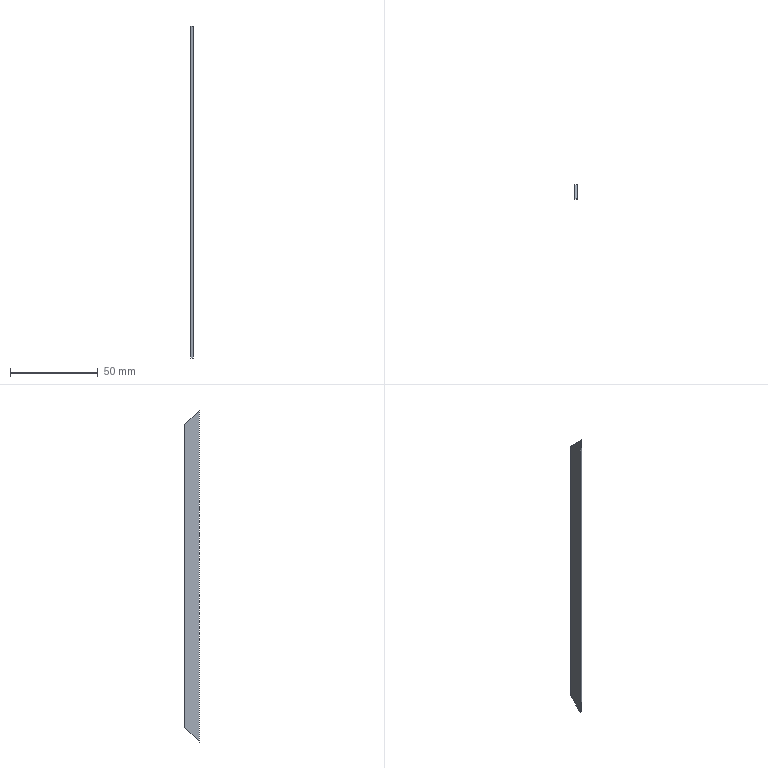Part | NX | features BREP 1 | 1 solid | 6 faces | box 1.5 x 8 x 189.5 mm | volume 2178 mm3 | plane 6
STEP:
#1=CARTESIAN_POINT('',(0.,8.,86.75));
#2=VERTEX_POINT('',#1);
#3=CARTESIAN_POINT('',(0.,8.,-86.75));
#4=VERTEX_POINT('',#3);
#5=CARTESIAN_POINT('',(0.,8.,94.75));
#6=DIRECTION('',(0.,0.,-1.));
#7=VECTOR('',#6,1000.);
#8=LINE('',#5,#7);
#9=EDGE_CURVE('',#2,#4,#8,.T.);
#10=ORIENTED_EDGE('',*,*,#9,.T.);
#11=CARTESIAN_POINT('',(0.,0.,-94.75));
#12=VERTEX_POINT('',#11);
#13=CARTESIAN_POINT('',(0.,8.,-86.75));
#14=DIRECTION('',(0.,-0.7071,-0.7071));
#15=VECTOR('',#14,1000.);
#16=LINE('',#13,#15);
#17=EDGE_CURVE('',#4,#12,#16,.T.);
#18=ORIENTED_EDGE('',*,*,#17,.T.);
#19=CARTESIAN_POINT('',(0.,0.,94.75));
#20=VERTEX_POINT('',#19);
#21=CARTESIAN_POINT('',(0.,0.,94.75));
#22=DIRECTION('',(0.,0.,-1.));
#23=VECTOR('',#22,1000.);
#24=LINE('',#21,#23);
#25=EDGE_CURVE('',#20,#12,#24,.T.);
#26=ORIENTED_EDGE('',*,*,#25,.F.);
#27=CARTESIAN_POINT('',(0.,0.,94.75));
#28=DIRECTION('',(0.,0.7071,-0.7071));
#29=VECTOR('',#28,1000.);
#30=LINE('',#27,#29);
#31=EDGE_CURVE('',#20,#2,#30,.T.);
#32=ORIENTED_EDGE('',*,*,#31,.T.);
#33=EDGE_LOOP('',(#10,#18,#26,#32));
#34=FACE_BOUND('',#33,.T.);
#35=CARTESIAN_POINT('',(0.,0.,94.75));
#36=DIRECTION('',(1.,0.,0.));
#37=DIRECTION('',(0.,1.,0.));
#38=AXIS2_PLACEMENT_3D('',#35,#36,#37);
#39=PLANE('',#38);
#40=ADVANCED_FACE('',(#34),#39,.F.);
#41=CARTESIAN_POINT('',(1.5,0.,-94.75));
#42=VERTEX_POINT('',#41);
#43=CARTESIAN_POINT('',(0.,0.,-94.75));
#44=DIRECTION('',(1.,0.,0.));
#45=VECTOR('',#44,1000.);
#46=LINE('',#43,#45);
#47=EDGE_CURVE('',#12,#42,#46,.T.);
#48=ORIENTED_EDGE('',*,*,#47,.T.);
#49=CARTESIAN_POINT('',(1.5,0.,94.75));
#50=VERTEX_POINT('',#49);
#51=CARTESIAN_POINT('',(1.5,0.,94.75));
#52=DIRECTION('',(0.,0.,-1.));
#53=VECTOR('',#52,1000.);
#54=LINE('',#51,#53);
#55=EDGE_CURVE('',#50,#42,#54,.T.);
#56=ORIENTED_EDGE('',*,*,#55,.F.);
#57=CARTESIAN_POINT('',(0.,0.,94.75));
#58=DIRECTION('',(1.,0.,0.));
#59=VECTOR('',#58,1000.);
#60=LINE('',#57,#59);
#61=EDGE_CURVE('',#20,#50,#60,.T.);
#62=ORIENTED_EDGE('',*,*,#61,.F.);
#63=ORIENTED_EDGE('',*,*,#25,.T.);
#64=EDGE_LOOP('',(#48,#56,#62,#63));
#65=FACE_BOUND('',#64,.T.);
#66=CARTESIAN_POINT('',(0.,0.,94.75));
#67=DIRECTION('',(0.,1.,0.));
#68=DIRECTION('',(1.,0.,0.));
#69=AXIS2_PLACEMENT_3D('',#66,#67,#68);
#70=PLANE('',#69);
#71=ADVANCED_FACE('',(#65),#70,.F.);
#72=ORIENTED_EDGE('',*,*,#55,.T.);
#73=CARTESIAN_POINT('',(1.5,8.,-86.75));
#74=VERTEX_POINT('',#73);
#75=CARTESIAN_POINT('',(1.5,8.,-86.75));
#76=DIRECTION('',(0.,0.7071,0.7071));
#77=VECTOR('',#76,1000.);
#78=LINE('',#75,#77);
#79=EDGE_CURVE('',#42,#74,#78,.T.);
#80=ORIENTED_EDGE('',*,*,#79,.T.);
#81=CARTESIAN_POINT('',(1.5,8.,86.75));
#82=VERTEX_POINT('',#81);
#83=CARTESIAN_POINT('',(1.5,8.,94.75));
#84=DIRECTION('',(0.,0.,-1.));
#85=VECTOR('',#84,1000.);
#86=LINE('',#83,#85);
#87=EDGE_CURVE('',#82,#74,#86,.T.);
#88=ORIENTED_EDGE('',*,*,#87,.F.);
#89=CARTESIAN_POINT('',(1.5,0.,94.75));
#90=DIRECTION('',(0.,-0.7071,0.7071));
#91=VECTOR('',#90,1000.);
#92=LINE('',#89,#91);
#93=EDGE_CURVE('',#82,#50,#92,.T.);
#94=ORIENTED_EDGE('',*,*,#93,.T.);
#95=EDGE_LOOP('',(#72,#80,#88,#94));
#96=FACE_BOUND('',#95,.T.);
#97=CARTESIAN_POINT('',(1.5,0.,94.75));
#98=DIRECTION('',(-1.,0.,0.));
#99=DIRECTION('',(0.,0.,1.));
#100=AXIS2_PLACEMENT_3D('',#97,#98,#99);
#101=PLANE('',#100);
#102=ADVANCED_FACE('',(#96),#101,.F.);
#103=ORIENTED_EDGE('',*,*,#87,.T.);
#104=CARTESIAN_POINT('',(0.,8.,-86.75));
#105=DIRECTION('',(-1.,0.,0.));
#106=VECTOR('',#105,1000.);
#107=LINE('',#104,#106);
#108=EDGE_CURVE('',#74,#4,#107,.T.);
#109=ORIENTED_EDGE('',*,*,#108,.T.);
#110=ORIENTED_EDGE('',*,*,#9,.F.);
#111=CARTESIAN_POINT('',(0.,8.,86.75));
#112=DIRECTION('',(1.,0.,0.));
#113=VECTOR('',#112,1000.);
#114=LINE('',#111,#113);
#115=EDGE_CURVE('',#2,#82,#114,.T.);
#116=ORIENTED_EDGE('',*,*,#115,.T.);
#117=EDGE_LOOP('',(#103,#109,#110,#116));
#118=FACE_BOUND('',#117,.T.);
#119=CARTESIAN_POINT('',(0.,8.,94.75));
#120=DIRECTION('',(0.,-1.,0.));
#121=DIRECTION('',(0.,0.,-1.));
#122=AXIS2_PLACEMENT_3D('',#119,#120,#121);
#123=PLANE('',#122);
#124=ADVANCED_FACE('',(#118),#123,.F.);
#125=ORIENTED_EDGE('',*,*,#79,.F.);
#126=ORIENTED_EDGE('',*,*,#47,.F.);
#127=ORIENTED_EDGE('',*,*,#17,.F.);
#128=ORIENTED_EDGE('',*,*,#108,.F.);
#129=EDGE_LOOP('',(#125,#126,#127,#128));
#130=FACE_BOUND('',#129,.T.);
#131=CARTESIAN_POINT('',(0.,8.,-86.75));
#132=DIRECTION('',(0.,0.7071,-0.7071));
#133=DIRECTION('',(-1.,0.,0.));
#134=AXIS2_PLACEMENT_3D('',#131,#132,#133);
#135=PLANE('',#134);
#136=ADVANCED_FACE('',(#130),#135,.T.);
#137=ORIENTED_EDGE('',*,*,#93,.F.);
#138=ORIENTED_EDGE('',*,*,#115,.F.);
#139=ORIENTED_EDGE('',*,*,#31,.F.);
#140=ORIENTED_EDGE('',*,*,#61,.T.);
#141=EDGE_LOOP('',(#137,#138,#139,#140));
#142=FACE_BOUND('',#141,.T.);
#143=CARTESIAN_POINT('',(0.,0.,94.75));
#144=DIRECTION('',(0.,-0.7071,-0.7071));
#145=DIRECTION('',(0.,0.7071,-0.7071));
#146=AXIS2_PLACEMENT_3D('',#143,#144,#145);
#147=PLANE('',#146);
#148=ADVANCED_FACE('',(#142),#147,.F.);
#149=CLOSED_SHELL('',(#40,#71,#102,#124,#136,#148));
#150=MANIFOLD_SOLID_BREP('',#149);
#151=(LENGTH_UNIT()NAMED_UNIT(*)SI_UNIT(.MILLI.,.METRE.));
#152=UNCERTAINTY_MEASURE_WITH_UNIT(LENGTH_MEASURE(0.00001),#151,'','');
#153=(NAMED_UNIT(*)PLANE_ANGLE_UNIT()SI_UNIT($,.RADIAN.));
#154=(NAMED_UNIT(*)SI_UNIT($,.STERADIAN.)SOLID_ANGLE_UNIT());
#155=(GEOMETRIC_REPRESENTATION_CONTEXT(3)GLOBAL_UNCERTAINTY_ASSIGNED_CONTEXT((#152))GLOBAL_UNIT_ASSIGNED_CONTEXT((#151,#153,#154))REPRESENTATION_CONTEXT('',''));
#156=ADVANCED_BREP_SHAPE_REPRESENTATION('',(#150),#155);